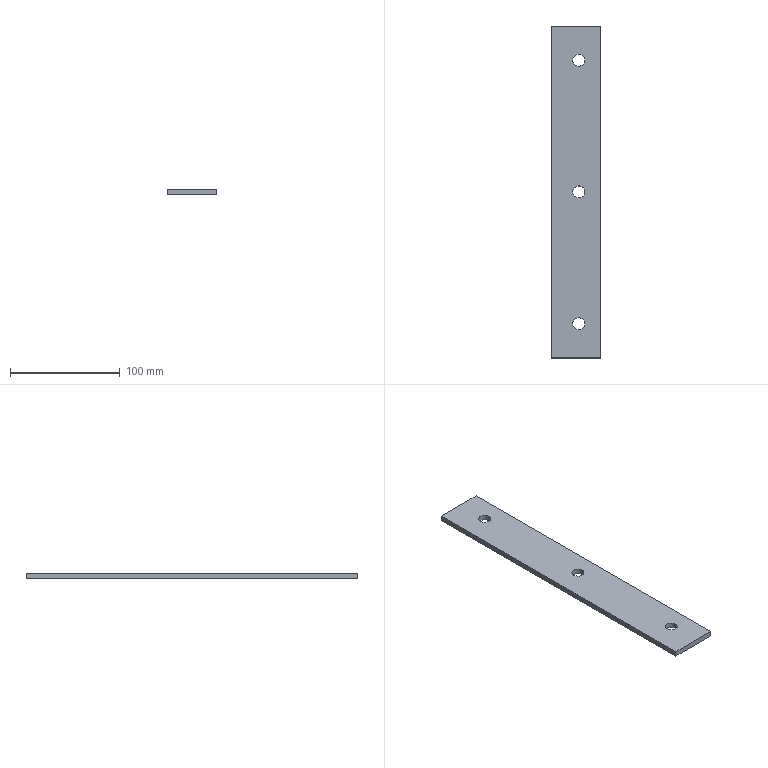Part | SolidWorks | features BaseBody 1 | 1 solid | 12 faces | box 45 x 302 x 5 mm | volume 66525 mm3 | cylinder 6 | plane 6 | commonest cylinder face diameters 11 x6
STEP:
#1=CARTESIAN_POINT('',(916.446,-3675.973,2072.471));
#2=VERTEX_POINT('',#1);
#3=CARTESIAN_POINT('',(927.446,-3675.973,2072.471));
#4=VERTEX_POINT('',#3);
#5=CARTESIAN_POINT('',(921.946,-3675.973,2072.471));
#6=DIRECTION('',(0.,0.,1.));
#7=DIRECTION('',(-1.,0.,0.));
#8=AXIS2_PLACEMENT_3D('',#5,#6,#7);
#9=CIRCLE('',#8,5.5);
#10=EDGE_CURVE('',#2,#4,#9,.T.);
#11=ORIENTED_EDGE('',*,*,#10,.T.);
#12=CARTESIAN_POINT('',(927.446,-3675.973,2067.471));
#13=VERTEX_POINT('',#12);
#14=CARTESIAN_POINT('',(927.446,-3675.973,2072.471));
#15=DIRECTION('',(0.,0.,-1.));
#16=VECTOR('',#15,1000.);
#17=LINE('',#14,#16);
#18=EDGE_CURVE('',#4,#13,#17,.T.);
#19=ORIENTED_EDGE('',*,*,#18,.T.);
#20=CARTESIAN_POINT('',(916.446,-3675.973,2067.471));
#21=VERTEX_POINT('',#20);
#22=CARTESIAN_POINT('',(921.946,-3675.973,2067.471));
#23=DIRECTION('',(0.,0.,-1.));
#24=DIRECTION('',(-1.,0.,0.));
#25=AXIS2_PLACEMENT_3D('',#22,#23,#24);
#26=CIRCLE('',#25,5.5);
#27=EDGE_CURVE('',#13,#21,#26,.T.);
#28=ORIENTED_EDGE('',*,*,#27,.T.);
#29=CARTESIAN_POINT('',(916.446,-3675.973,2072.471));
#30=DIRECTION('',(0.,0.,-1.));
#31=VECTOR('',#30,1000.);
#32=LINE('',#29,#31);
#33=EDGE_CURVE('',#2,#21,#32,.T.);
#34=ORIENTED_EDGE('',*,*,#33,.F.);
#35=EDGE_LOOP('',(#11,#19,#28,#34));
#36=FACE_OUTER_BOUND('',#35,.T.);
#37=CARTESIAN_POINT('',(921.946,-3675.973,2072.471));
#38=DIRECTION('',(0.,0.,-1.));
#39=DIRECTION('',(-1.,0.,0.));
#40=AXIS2_PLACEMENT_3D('',#37,#38,#39);
#41=CYLINDRICAL_SURFACE('',#40,5.5);
#42=ADVANCED_FACE('',(#36),#41,.F.);
#43=CARTESIAN_POINT('',(916.446,-3915.973,2072.471));
#44=VERTEX_POINT('',#43);
#45=CARTESIAN_POINT('',(927.446,-3915.973,2072.471));
#46=VERTEX_POINT('',#45);
#47=CARTESIAN_POINT('',(921.946,-3915.973,2072.471));
#48=DIRECTION('',(0.,0.,1.));
#49=DIRECTION('',(-1.,0.,0.));
#50=AXIS2_PLACEMENT_3D('',#47,#48,#49);
#51=CIRCLE('',#50,5.5);
#52=EDGE_CURVE('',#44,#46,#51,.T.);
#53=ORIENTED_EDGE('',*,*,#52,.T.);
#54=CARTESIAN_POINT('',(927.446,-3915.973,2067.471));
#55=VERTEX_POINT('',#54);
#56=CARTESIAN_POINT('',(927.446,-3915.973,2072.471));
#57=DIRECTION('',(0.,0.,-1.));
#58=VECTOR('',#57,1000.);
#59=LINE('',#56,#58);
#60=EDGE_CURVE('',#46,#55,#59,.T.);
#61=ORIENTED_EDGE('',*,*,#60,.T.);
#62=CARTESIAN_POINT('',(916.446,-3915.973,2067.471));
#63=VERTEX_POINT('',#62);
#64=CARTESIAN_POINT('',(921.946,-3915.973,2067.471));
#65=DIRECTION('',(0.,0.,-1.));
#66=DIRECTION('',(-1.,0.,0.));
#67=AXIS2_PLACEMENT_3D('',#64,#65,#66);
#68=CIRCLE('',#67,5.5);
#69=EDGE_CURVE('',#55,#63,#68,.T.);
#70=ORIENTED_EDGE('',*,*,#69,.T.);
#71=CARTESIAN_POINT('',(916.446,-3915.973,2072.471));
#72=DIRECTION('',(0.,0.,-1.));
#73=VECTOR('',#72,1000.);
#74=LINE('',#71,#73);
#75=EDGE_CURVE('',#44,#63,#74,.T.);
#76=ORIENTED_EDGE('',*,*,#75,.F.);
#77=EDGE_LOOP('',(#53,#61,#70,#76));
#78=FACE_OUTER_BOUND('',#77,.T.);
#79=CARTESIAN_POINT('',(921.946,-3915.973,2072.471));
#80=DIRECTION('',(0.,0.,-1.));
#81=DIRECTION('',(-1.,0.,0.));
#82=AXIS2_PLACEMENT_3D('',#79,#80,#81);
#83=CYLINDRICAL_SURFACE('',#82,5.5);
#84=ADVANCED_FACE('',(#78),#83,.F.);
#85=CARTESIAN_POINT('',(916.446,-3795.973,2072.471));
#86=VERTEX_POINT('',#85);
#87=CARTESIAN_POINT('',(927.446,-3795.973,2072.471));
#88=VERTEX_POINT('',#87);
#89=CARTESIAN_POINT('',(921.946,-3795.973,2072.471));
#90=DIRECTION('',(0.,0.,1.));
#91=DIRECTION('',(-1.,0.,0.));
#92=AXIS2_PLACEMENT_3D('',#89,#90,#91);
#93=CIRCLE('',#92,5.5);
#94=EDGE_CURVE('',#86,#88,#93,.T.);
#95=ORIENTED_EDGE('',*,*,#94,.T.);
#96=CARTESIAN_POINT('',(927.446,-3795.973,2067.471));
#97=VERTEX_POINT('',#96);
#98=CARTESIAN_POINT('',(927.446,-3795.973,2072.471));
#99=DIRECTION('',(0.,0.,-1.));
#100=VECTOR('',#99,1000.);
#101=LINE('',#98,#100);
#102=EDGE_CURVE('',#88,#97,#101,.T.);
#103=ORIENTED_EDGE('',*,*,#102,.T.);
#104=CARTESIAN_POINT('',(916.446,-3795.973,2067.471));
#105=VERTEX_POINT('',#104);
#106=CARTESIAN_POINT('',(921.946,-3795.973,2067.471));
#107=DIRECTION('',(0.,0.,-1.));
#108=DIRECTION('',(-1.,0.,0.));
#109=AXIS2_PLACEMENT_3D('',#106,#107,#108);
#110=CIRCLE('',#109,5.5);
#111=EDGE_CURVE('',#97,#105,#110,.T.);
#112=ORIENTED_EDGE('',*,*,#111,.T.);
#113=CARTESIAN_POINT('',(916.446,-3795.973,2072.471));
#114=DIRECTION('',(0.,0.,-1.));
#115=VECTOR('',#114,1000.);
#116=LINE('',#113,#115);
#117=EDGE_CURVE('',#86,#105,#116,.T.);
#118=ORIENTED_EDGE('',*,*,#117,.F.);
#119=EDGE_LOOP('',(#95,#103,#112,#118));
#120=FACE_OUTER_BOUND('',#119,.T.);
#121=CARTESIAN_POINT('',(921.946,-3795.973,2072.471));
#122=DIRECTION('',(0.,0.,-1.));
#123=DIRECTION('',(-1.,0.,0.));
#124=AXIS2_PLACEMENT_3D('',#121,#122,#123);
#125=CYLINDRICAL_SURFACE('',#124,5.5);
#126=ADVANCED_FACE('',(#120),#125,.F.);
#127=CARTESIAN_POINT('',(896.946,-3644.973,2067.471));
#128=VERTEX_POINT('',#127);
#129=CARTESIAN_POINT('',(896.946,-3946.973,2067.471));
#130=VERTEX_POINT('',#129);
#131=CARTESIAN_POINT('',(896.946,-3795.973,2067.471));
#132=DIRECTION('',(0.,-1.,0.));
#133=VECTOR('',#132,1000.);
#134=LINE('',#131,#133);
#135=EDGE_CURVE('',#128,#130,#134,.T.);
#136=ORIENTED_EDGE('',*,*,#135,.F.);
#137=CARTESIAN_POINT('',(941.946,-3644.973,2067.471));
#138=VERTEX_POINT('',#137);
#139=CARTESIAN_POINT('',(919.446,-3644.973,2067.471));
#140=DIRECTION('',(-1.,0.,0.));
#141=VECTOR('',#140,1000.);
#142=LINE('',#139,#141);
#143=EDGE_CURVE('',#138,#128,#142,.T.);
#144=ORIENTED_EDGE('',*,*,#143,.F.);
#145=CARTESIAN_POINT('',(941.946,-3946.973,2067.471));
#146=VERTEX_POINT('',#145);
#147=CARTESIAN_POINT('',(941.946,-3795.973,2067.471));
#148=DIRECTION('',(0.,1.,0.));
#149=VECTOR('',#148,1000.);
#150=LINE('',#147,#149);
#151=EDGE_CURVE('',#146,#138,#150,.T.);
#152=ORIENTED_EDGE('',*,*,#151,.F.);
#153=CARTESIAN_POINT('',(919.446,-3946.973,2067.471));
#154=DIRECTION('',(1.,0.,0.));
#155=VECTOR('',#154,1000.);
#156=LINE('',#153,#155);
#157=EDGE_CURVE('',#130,#146,#156,.T.);
#158=ORIENTED_EDGE('',*,*,#157,.F.);
#159=EDGE_LOOP('',(#136,#144,#152,#158));
#160=FACE_OUTER_BOUND('',#159,.T.);
#161=CARTESIAN_POINT('',(921.946,-3675.973,2067.471));
#162=DIRECTION('',(0.,0.,-1.));
#163=DIRECTION('',(-1.,0.,0.));
#164=AXIS2_PLACEMENT_3D('',#161,#162,#163);
#165=CIRCLE('',#164,5.5);
#166=EDGE_CURVE('',#21,#13,#165,.T.);
#167=ORIENTED_EDGE('',*,*,#166,.F.);
#168=ORIENTED_EDGE('',*,*,#27,.F.);
#169=EDGE_LOOP('',(#167,#168));
#170=FACE_BOUND('',#169,.T.);
#171=CARTESIAN_POINT('',(921.946,-3915.973,2067.471));
#172=DIRECTION('',(0.,0.,-1.));
#173=DIRECTION('',(-1.,0.,0.));
#174=AXIS2_PLACEMENT_3D('',#171,#172,#173);
#175=CIRCLE('',#174,5.5);
#176=EDGE_CURVE('',#63,#55,#175,.T.);
#177=ORIENTED_EDGE('',*,*,#176,.F.);
#178=ORIENTED_EDGE('',*,*,#69,.F.);
#179=EDGE_LOOP('',(#177,#178));
#180=FACE_BOUND('',#179,.T.);
#181=CARTESIAN_POINT('',(921.946,-3795.973,2067.471));
#182=DIRECTION('',(0.,0.,-1.));
#183=DIRECTION('',(-1.,0.,0.));
#184=AXIS2_PLACEMENT_3D('',#181,#182,#183);
#185=CIRCLE('',#184,5.5);
#186=EDGE_CURVE('',#105,#97,#185,.T.);
#187=ORIENTED_EDGE('',*,*,#186,.F.);
#188=ORIENTED_EDGE('',*,*,#111,.F.);
#189=EDGE_LOOP('',(#187,#188));
#190=FACE_BOUND('',#189,.T.);
#191=CARTESIAN_POINT('',(919.446,-3795.973,2067.471));
#192=DIRECTION('',(0.,0.,1.));
#193=DIRECTION('',(1.,0.,0.));
#194=AXIS2_PLACEMENT_3D('',#191,#192,#193);
#195=PLANE('',#194);
#196=ADVANCED_FACE('',(#160,#170,#180,#190),#195,.F.);
#197=ORIENTED_EDGE('',*,*,#157,.T.);
#198=CARTESIAN_POINT('',(941.946,-3946.973,2072.471));
#199=VERTEX_POINT('',#198);
#200=CARTESIAN_POINT('',(941.946,-3946.973,2067.471));
#201=DIRECTION('',(0.,0.,1.));
#202=VECTOR('',#201,1000.);
#203=LINE('',#200,#202);
#204=EDGE_CURVE('',#146,#199,#203,.T.);
#205=ORIENTED_EDGE('',*,*,#204,.T.);
#206=CARTESIAN_POINT('',(896.946,-3946.973,2072.471));
#207=VERTEX_POINT('',#206);
#208=CARTESIAN_POINT('',(896.946,-3946.973,2072.471));
#209=DIRECTION('',(-1.,0.,0.));
#210=VECTOR('',#209,1000.);
#211=LINE('',#208,#210);
#212=EDGE_CURVE('',#199,#207,#211,.T.);
#213=ORIENTED_EDGE('',*,*,#212,.T.);
#214=CARTESIAN_POINT('',(896.946,-3946.973,2067.471));
#215=DIRECTION('',(0.,0.,-1.));
#216=VECTOR('',#215,1000.);
#217=LINE('',#214,#216);
#218=EDGE_CURVE('',#207,#130,#217,.T.);
#219=ORIENTED_EDGE('',*,*,#218,.T.);
#220=EDGE_LOOP('',(#197,#205,#213,#219));
#221=FACE_OUTER_BOUND('',#220,.T.);
#222=CARTESIAN_POINT('',(896.946,-3946.973,2067.471));
#223=DIRECTION('',(0.,-1.,0.));
#224=DIRECTION('',(0.,0.,-1.));
#225=AXIS2_PLACEMENT_3D('',#222,#223,#224);
#226=PLANE('',#225);
#227=ADVANCED_FACE('',(#221),#226,.T.);
#228=ORIENTED_EDGE('',*,*,#135,.T.);
#229=ORIENTED_EDGE('',*,*,#218,.F.);
#230=CARTESIAN_POINT('',(896.946,-3644.973,2072.471));
#231=VERTEX_POINT('',#230);
#232=CARTESIAN_POINT('',(896.946,-3644.973,2072.471));
#233=DIRECTION('',(0.,1.,0.));
#234=VECTOR('',#233,1000.);
#235=LINE('',#232,#234);
#236=EDGE_CURVE('',#207,#231,#235,.T.);
#237=ORIENTED_EDGE('',*,*,#236,.T.);
#238=CARTESIAN_POINT('',(896.946,-3644.973,2067.471));
#239=DIRECTION('',(0.,0.,-1.));
#240=VECTOR('',#239,1000.);
#241=LINE('',#238,#240);
#242=EDGE_CURVE('',#231,#128,#241,.T.);
#243=ORIENTED_EDGE('',*,*,#242,.T.);
#244=EDGE_LOOP('',(#228,#229,#237,#243));
#245=FACE_OUTER_BOUND('',#244,.T.);
#246=CARTESIAN_POINT('',(896.946,-3644.973,2067.471));
#247=DIRECTION('',(-1.,0.,0.));
#248=DIRECTION('',(0.,0.,1.));
#249=AXIS2_PLACEMENT_3D('',#246,#247,#248);
#250=PLANE('',#249);
#251=ADVANCED_FACE('',(#245),#250,.T.);
#252=ORIENTED_EDGE('',*,*,#143,.T.);
#253=ORIENTED_EDGE('',*,*,#242,.F.);
#254=CARTESIAN_POINT('',(941.946,-3644.973,2072.471));
#255=VERTEX_POINT('',#254);
#256=CARTESIAN_POINT('',(941.946,-3644.973,2072.471));
#257=DIRECTION('',(1.,0.,0.));
#258=VECTOR('',#257,1000.);
#259=LINE('',#256,#258);
#260=EDGE_CURVE('',#231,#255,#259,.T.);
#261=ORIENTED_EDGE('',*,*,#260,.T.);
#262=CARTESIAN_POINT('',(941.946,-3644.973,2067.471));
#263=DIRECTION('',(0.,0.,-1.));
#264=VECTOR('',#263,1000.);
#265=LINE('',#262,#264);
#266=EDGE_CURVE('',#255,#138,#265,.T.);
#267=ORIENTED_EDGE('',*,*,#266,.T.);
#268=EDGE_LOOP('',(#252,#253,#261,#267));
#269=FACE_OUTER_BOUND('',#268,.T.);
#270=CARTESIAN_POINT('',(941.946,-3644.973,2067.471));
#271=DIRECTION('',(0.,1.,0.));
#272=DIRECTION('',(0.,0.,1.));
#273=AXIS2_PLACEMENT_3D('',#270,#271,#272);
#274=PLANE('',#273);
#275=ADVANCED_FACE('',(#269),#274,.T.);
#276=ORIENTED_EDGE('',*,*,#151,.T.);
#277=ORIENTED_EDGE('',*,*,#266,.F.);
#278=CARTESIAN_POINT('',(941.946,-3946.973,2072.471));
#279=DIRECTION('',(0.,-1.,0.));
#280=VECTOR('',#279,1000.);
#281=LINE('',#278,#280);
#282=EDGE_CURVE('',#255,#199,#281,.T.);
#283=ORIENTED_EDGE('',*,*,#282,.T.);
#284=ORIENTED_EDGE('',*,*,#204,.F.);
#285=EDGE_LOOP('',(#276,#277,#283,#284));
#286=FACE_OUTER_BOUND('',#285,.T.);
#287=CARTESIAN_POINT('',(941.946,-3946.973,2067.471));
#288=DIRECTION('',(1.,0.,0.));
#289=DIRECTION('',(0.,0.,-1.));
#290=AXIS2_PLACEMENT_3D('',#287,#288,#289);
#291=PLANE('',#290);
#292=ADVANCED_FACE('',(#286),#291,.T.);
#293=ORIENTED_EDGE('',*,*,#18,.F.);
#294=CARTESIAN_POINT('',(921.946,-3675.973,2072.471));
#295=DIRECTION('',(0.,0.,1.));
#296=DIRECTION('',(-1.,0.,0.));
#297=AXIS2_PLACEMENT_3D('',#294,#295,#296);
#298=CIRCLE('',#297,5.5);
#299=EDGE_CURVE('',#4,#2,#298,.T.);
#300=ORIENTED_EDGE('',*,*,#299,.T.);
#301=ORIENTED_EDGE('',*,*,#33,.T.);
#302=ORIENTED_EDGE('',*,*,#166,.T.);
#303=EDGE_LOOP('',(#293,#300,#301,#302));
#304=FACE_OUTER_BOUND('',#303,.T.);
#305=CARTESIAN_POINT('',(921.946,-3675.973,2072.471));
#306=DIRECTION('',(0.,0.,-1.));
#307=DIRECTION('',(-1.,0.,0.));
#308=AXIS2_PLACEMENT_3D('',#305,#306,#307);
#309=CYLINDRICAL_SURFACE('',#308,5.5);
#310=ADVANCED_FACE('',(#304),#309,.F.);
#311=ORIENTED_EDGE('',*,*,#60,.F.);
#312=CARTESIAN_POINT('',(921.946,-3915.973,2072.471));
#313=DIRECTION('',(0.,0.,1.));
#314=DIRECTION('',(-1.,0.,0.));
#315=AXIS2_PLACEMENT_3D('',#312,#313,#314);
#316=CIRCLE('',#315,5.5);
#317=EDGE_CURVE('',#46,#44,#316,.T.);
#318=ORIENTED_EDGE('',*,*,#317,.T.);
#319=ORIENTED_EDGE('',*,*,#75,.T.);
#320=ORIENTED_EDGE('',*,*,#176,.T.);
#321=EDGE_LOOP('',(#311,#318,#319,#320));
#322=FACE_OUTER_BOUND('',#321,.T.);
#323=CARTESIAN_POINT('',(921.946,-3915.973,2072.471));
#324=DIRECTION('',(0.,0.,-1.));
#325=DIRECTION('',(-1.,0.,0.));
#326=AXIS2_PLACEMENT_3D('',#323,#324,#325);
#327=CYLINDRICAL_SURFACE('',#326,5.5);
#328=ADVANCED_FACE('',(#322),#327,.F.);
#329=ORIENTED_EDGE('',*,*,#102,.F.);
#330=CARTESIAN_POINT('',(921.946,-3795.973,2072.471));
#331=DIRECTION('',(0.,0.,1.));
#332=DIRECTION('',(-1.,0.,0.));
#333=AXIS2_PLACEMENT_3D('',#330,#331,#332);
#334=CIRCLE('',#333,5.5);
#335=EDGE_CURVE('',#88,#86,#334,.T.);
#336=ORIENTED_EDGE('',*,*,#335,.T.);
#337=ORIENTED_EDGE('',*,*,#117,.T.);
#338=ORIENTED_EDGE('',*,*,#186,.T.);
#339=EDGE_LOOP('',(#329,#336,#337,#338));
#340=FACE_OUTER_BOUND('',#339,.T.);
#341=CARTESIAN_POINT('',(921.946,-3795.973,2072.471));
#342=DIRECTION('',(0.,0.,-1.));
#343=DIRECTION('',(-1.,0.,0.));
#344=AXIS2_PLACEMENT_3D('',#341,#342,#343);
#345=CYLINDRICAL_SURFACE('',#344,5.5);
#346=ADVANCED_FACE('',(#340),#345,.F.);
#347=ORIENTED_EDGE('',*,*,#236,.F.);
#348=ORIENTED_EDGE('',*,*,#212,.F.);
#349=ORIENTED_EDGE('',*,*,#282,.F.);
#350=ORIENTED_EDGE('',*,*,#260,.F.);
#351=EDGE_LOOP('',(#347,#348,#349,#350));
#352=FACE_OUTER_BOUND('',#351,.T.);
#353=ORIENTED_EDGE('',*,*,#10,.F.);
#354=ORIENTED_EDGE('',*,*,#299,.F.);
#355=EDGE_LOOP('',(#353,#354));
#356=FACE_BOUND('',#355,.T.);
#357=ORIENTED_EDGE('',*,*,#52,.F.);
#358=ORIENTED_EDGE('',*,*,#317,.F.);
#359=EDGE_LOOP('',(#357,#358));
#360=FACE_BOUND('',#359,.T.);
#361=ORIENTED_EDGE('',*,*,#94,.F.);
#362=ORIENTED_EDGE('',*,*,#335,.F.);
#363=EDGE_LOOP('',(#361,#362));
#364=FACE_BOUND('',#363,.T.);
#365=CARTESIAN_POINT('',(919.446,-3795.973,2072.471));
#366=DIRECTION('',(0.,0.,1.));
#367=DIRECTION('',(1.,0.,0.));
#368=AXIS2_PLACEMENT_3D('',#365,#366,#367);
#369=PLANE('',#368);
#370=ADVANCED_FACE('',(#352,#356,#360,#364),#369,.T.);
#371=CLOSED_SHELL('',(#42,#84,#126,#196,#227,#251,#275,#292,#310,#328,#346,#370));
#372=MANIFOLD_SOLID_BREP('',#371);
#373=CARTESIAN_POINT('',(0.,0.,0.));
#374=DIRECTION('',(0.,0.,1.));
#375=DIRECTION('',(1.,0.,0.));
#376=AXIS2_PLACEMENT_3D('',#373,#374,#375);
#377=(LENGTH_UNIT()NAMED_UNIT(*)SI_UNIT(.MILLI.,.METRE.));
#378=UNCERTAINTY_MEASURE_WITH_UNIT(LENGTH_MEASURE(0.00001),#377,'','');
#379=(NAMED_UNIT(*)PLANE_ANGLE_UNIT()SI_UNIT($,.RADIAN.));
#380=(NAMED_UNIT(*)SI_UNIT($,.STERADIAN.)SOLID_ANGLE_UNIT());
#381=(GEOMETRIC_REPRESENTATION_CONTEXT(3)GLOBAL_UNCERTAINTY_ASSIGNED_CONTEXT((#378))GLOBAL_UNIT_ASSIGNED_CONTEXT((#377,#379,#380))REPRESENTATION_CONTEXT('',''));
#382=ADVANCED_BREP_SHAPE_REPRESENTATION('',(#372,#376),#381);